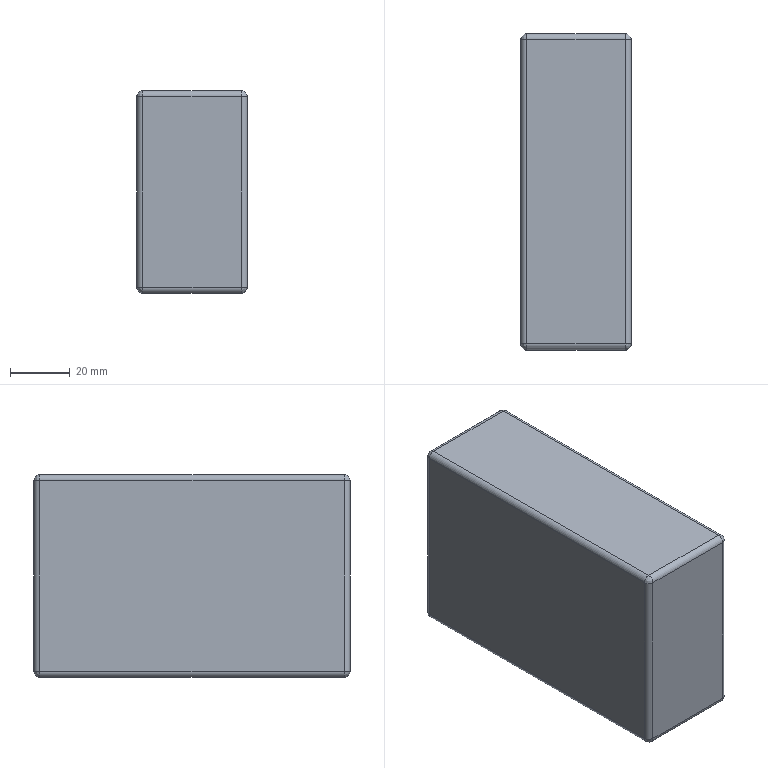Part | SolidWorks | features BaseBody 1 | 1 solid | 26 faces | box 37 x 106 x 68 mm | volume 265982 mm3 | cylinder 12 | spline 8 | plane 6 | commonest cylinder face diameters 4 x12
STEP:
#1=CARTESIAN_POINT('',(-18.5,-51.,-32.));
#2=VERTEX_POINT('',#1);
#3=CARTESIAN_POINT('',(-18.5,51.,-32.));
#4=VERTEX_POINT('',#3);
#5=CARTESIAN_POINT('',(-18.5,53.,-32.));
#6=DIRECTION('',(0.,1.,0.));
#7=VECTOR('',#6,1000.);
#8=LINE('',#5,#7);
#9=EDGE_CURVE('',#2,#4,#8,.T.);
#10=ORIENTED_EDGE('',*,*,#9,.F.);
#11=CARTESIAN_POINT('',(-18.5,-51.,32.));
#12=VERTEX_POINT('',#11);
#13=CARTESIAN_POINT('',(-18.5,-51.,-34.));
#14=DIRECTION('',(0.,0.,-1.));
#15=VECTOR('',#14,1000.);
#16=LINE('',#13,#15);
#17=EDGE_CURVE('',#12,#2,#16,.T.);
#18=ORIENTED_EDGE('',*,*,#17,.F.);
#19=CARTESIAN_POINT('',(-18.5,51.,32.));
#20=VERTEX_POINT('',#19);
#21=CARTESIAN_POINT('',(-18.5,53.,32.));
#22=DIRECTION('',(0.,-1.,0.));
#23=VECTOR('',#22,1000.);
#24=LINE('',#21,#23);
#25=EDGE_CURVE('',#20,#12,#24,.T.);
#26=ORIENTED_EDGE('',*,*,#25,.F.);
#27=CARTESIAN_POINT('',(-18.5,51.,-34.));
#28=DIRECTION('',(0.,0.,1.));
#29=VECTOR('',#28,1000.);
#30=LINE('',#27,#29);
#31=EDGE_CURVE('',#4,#20,#30,.T.);
#32=ORIENTED_EDGE('',*,*,#31,.F.);
#33=EDGE_LOOP('',(#10,#18,#26,#32));
#34=FACE_OUTER_BOUND('',#33,.T.);
#35=CARTESIAN_POINT('',(-18.5,53.,-34.));
#36=DIRECTION('',(1.,0.,0.));
#37=DIRECTION('',(0.,0.,-1.));
#38=AXIS2_PLACEMENT_3D('',#35,#36,#37);
#39=PLANE('',#38);
#40=ADVANCED_FACE('',(#34),#39,.F.);
#41=CARTESIAN_POINT('',(-16.5,53.,32.));
#42=VERTEX_POINT('',#41);
#43=CARTESIAN_POINT('',(-16.5,53.,-32.));
#44=VERTEX_POINT('',#43);
#45=CARTESIAN_POINT('',(-16.5,53.,0.));
#46=DIRECTION('',(0.,0.,-1.));
#47=VECTOR('',#46,1000.);
#48=LINE('',#45,#47);
#49=EDGE_CURVE('',#42,#44,#48,.T.);
#50=ORIENTED_EDGE('',*,*,#49,.T.);
#51=CARTESIAN_POINT('',(-16.5,51.,-32.));
#52=DIRECTION('',(0.,0.,1.));
#53=DIRECTION('',(1.,0.,0.));
#54=AXIS2_PLACEMENT_3D('',#51,#52,#53);
#55=CIRCLE('',#54,2.);
#56=EDGE_CURVE('',#44,#4,#55,.T.);
#57=ORIENTED_EDGE('',*,*,#56,.T.);
#58=ORIENTED_EDGE('',*,*,#31,.T.);
#59=CARTESIAN_POINT('',(-16.5,51.,32.));
#60=DIRECTION('',(0.,0.,-1.));
#61=DIRECTION('',(1.,0.,0.));
#62=AXIS2_PLACEMENT_3D('',#59,#60,#61);
#63=CIRCLE('',#62,2.);
#64=EDGE_CURVE('',#20,#42,#63,.T.);
#65=ORIENTED_EDGE('',*,*,#64,.T.);
#66=EDGE_LOOP('',(#50,#57,#58,#65));
#67=FACE_OUTER_BOUND('',#66,.T.);
#68=CARTESIAN_POINT('',(-16.5,51.,0.));
#69=DIRECTION('',(0.,0.,1.));
#70=DIRECTION('',(1.,0.,0.));
#71=AXIS2_PLACEMENT_3D('',#68,#69,#70);
#72=CYLINDRICAL_SURFACE('',#71,2.);
#73=ADVANCED_FACE('',(#67),#72,.T.);
#74=CARTESIAN_POINT('',(-16.5,51.,-34.));
#75=VERTEX_POINT('',#74);
#76=CARTESIAN_POINT('',(-16.5,51.,-32.));
#77=DIRECTION('',(0.,-1.,0.));
#78=DIRECTION('',(0.,0.,-1.));
#79=AXIS2_PLACEMENT_3D('',#76,#77,#78);
#80=CIRCLE('',#79,2.);
#81=EDGE_CURVE('',#4,#75,#80,.T.);
#82=ORIENTED_EDGE('',*,*,#81,.T.);
#83=CARTESIAN_POINT('',(-16.5,-51.,-34.));
#84=VERTEX_POINT('',#83);
#85=CARTESIAN_POINT('',(-16.5,53.,-34.));
#86=DIRECTION('',(0.,-1.,0.));
#87=VECTOR('',#86,1000.);
#88=LINE('',#85,#87);
#89=EDGE_CURVE('',#75,#84,#88,.T.);
#90=ORIENTED_EDGE('',*,*,#89,.T.);
#91=CARTESIAN_POINT('',(-16.5,-51.,-32.));
#92=DIRECTION('',(0.,1.,0.));
#93=DIRECTION('',(0.,0.,-1.));
#94=AXIS2_PLACEMENT_3D('',#91,#92,#93);
#95=CIRCLE('',#94,2.);
#96=EDGE_CURVE('',#84,#2,#95,.T.);
#97=ORIENTED_EDGE('',*,*,#96,.T.);
#98=ORIENTED_EDGE('',*,*,#9,.T.);
#99=EDGE_LOOP('',(#82,#90,#97,#98));
#100=FACE_OUTER_BOUND('',#99,.T.);
#101=CARTESIAN_POINT('',(-16.5,53.,-32.));
#102=DIRECTION('',(0.,-1.,0.));
#103=DIRECTION('',(0.,0.,-1.));
#104=AXIS2_PLACEMENT_3D('',#101,#102,#103);
#105=CYLINDRICAL_SURFACE('',#104,2.);
#106=ADVANCED_FACE('',(#100),#105,.T.);
#107=ORIENTED_EDGE('',*,*,#17,.T.);
#108=CARTESIAN_POINT('',(-16.5,-53.,-32.));
#109=VERTEX_POINT('',#108);
#110=CARTESIAN_POINT('',(-16.5,-51.,-32.));
#111=DIRECTION('',(0.,0.,1.));
#112=DIRECTION('',(-1.,0.,0.));
#113=AXIS2_PLACEMENT_3D('',#110,#111,#112);
#114=CIRCLE('',#113,2.);
#115=EDGE_CURVE('',#2,#109,#114,.T.);
#116=ORIENTED_EDGE('',*,*,#115,.T.);
#117=CARTESIAN_POINT('',(-16.5,-53.,32.));
#118=VERTEX_POINT('',#117);
#119=CARTESIAN_POINT('',(-16.5,-53.,-34.));
#120=DIRECTION('',(0.,0.,1.));
#121=VECTOR('',#120,1000.);
#122=LINE('',#119,#121);
#123=EDGE_CURVE('',#109,#118,#122,.T.);
#124=ORIENTED_EDGE('',*,*,#123,.T.);
#125=CARTESIAN_POINT('',(-16.5,-51.,32.));
#126=DIRECTION('',(0.,0.,-1.));
#127=DIRECTION('',(-1.,0.,0.));
#128=AXIS2_PLACEMENT_3D('',#125,#126,#127);
#129=CIRCLE('',#128,2.);
#130=EDGE_CURVE('',#118,#12,#129,.T.);
#131=ORIENTED_EDGE('',*,*,#130,.T.);
#132=EDGE_LOOP('',(#107,#116,#124,#131));
#133=FACE_OUTER_BOUND('',#132,.T.);
#134=CARTESIAN_POINT('',(-16.5,-51.,-34.));
#135=DIRECTION('',(0.,0.,-1.));
#136=DIRECTION('',(-1.,0.,0.));
#137=AXIS2_PLACEMENT_3D('',#134,#135,#136);
#138=CYLINDRICAL_SURFACE('',#137,2.);
#139=ADVANCED_FACE('',(#133),#138,.T.);
#140=CARTESIAN_POINT('',(-16.5,51.,34.));
#141=VERTEX_POINT('',#140);
#142=CARTESIAN_POINT('',(-16.5,51.,32.));
#143=DIRECTION('',(0.,-1.,0.));
#144=DIRECTION('',(0.,0.,-1.));
#145=AXIS2_PLACEMENT_3D('',#142,#143,#144);
#146=CIRCLE('',#145,2.);
#147=EDGE_CURVE('',#141,#20,#146,.T.);
#148=ORIENTED_EDGE('',*,*,#147,.T.);
#149=ORIENTED_EDGE('',*,*,#25,.T.);
#150=CARTESIAN_POINT('',(-16.5,-51.,34.));
#151=VERTEX_POINT('',#150);
#152=CARTESIAN_POINT('',(-16.5,-51.,32.));
#153=DIRECTION('',(0.,1.,0.));
#154=DIRECTION('',(0.,0.,-1.));
#155=AXIS2_PLACEMENT_3D('',#152,#153,#154);
#156=CIRCLE('',#155,2.);
#157=EDGE_CURVE('',#12,#151,#156,.T.);
#158=ORIENTED_EDGE('',*,*,#157,.T.);
#159=CARTESIAN_POINT('',(-16.5,53.,34.));
#160=DIRECTION('',(0.,1.,0.));
#161=VECTOR('',#160,1000.);
#162=LINE('',#159,#161);
#163=EDGE_CURVE('',#151,#141,#162,.T.);
#164=ORIENTED_EDGE('',*,*,#163,.T.);
#165=EDGE_LOOP('',(#148,#149,#158,#164));
#166=FACE_OUTER_BOUND('',#165,.T.);
#167=CARTESIAN_POINT('',(-16.5,53.,32.));
#168=DIRECTION('',(0.,-1.,0.));
#169=DIRECTION('',(0.,0.,-1.));
#170=AXIS2_PLACEMENT_3D('',#167,#168,#169);
#171=CYLINDRICAL_SURFACE('',#170,2.);
#172=ADVANCED_FACE('',(#166),#171,.T.);
#173=ORIENTED_EDGE('',*,*,#81,.F.);
#174=ORIENTED_EDGE('',*,*,#56,.F.);
#175=CARTESIAN_POINT('',(-16.5,51.,-32.));
#176=DIRECTION('',(-1.,0.,0.));
#177=DIRECTION('',(0.,0.,-1.));
#178=AXIS2_PLACEMENT_3D('',#175,#176,#177);
#179=CIRCLE('',#178,2.);
#180=EDGE_CURVE('',#44,#75,#179,.T.);
#181=ORIENTED_EDGE('',*,*,#180,.T.);
#182=EDGE_LOOP('',(#173,#174,#181));
#183=FACE_OUTER_BOUND('',#182,.T.);
#184=CARTESIAN_POINT('',(-16.5,51.,-34.));
#185=CARTESIAN_POINT('',(-16.5,51.,-34.));
#186=CARTESIAN_POINT('',(-16.5,51.,-34.));
#187=CARTESIAN_POINT('',(-16.5,51.,-34.));
#188=CARTESIAN_POINT('',(-17.672,51.,-34.));
#189=CARTESIAN_POINT('',(-17.672,51.686,-34.));
#190=CARTESIAN_POINT('',(-17.186,52.172,-34.));
#191=CARTESIAN_POINT('',(-16.5,52.172,-34.));
#192=CARTESIAN_POINT('',(-18.5,51.,-33.172));
#193=CARTESIAN_POINT('',(-18.5,52.172,-33.172));
#194=CARTESIAN_POINT('',(-17.672,53.,-33.172));
#195=CARTESIAN_POINT('',(-16.5,53.,-33.172));
#196=CARTESIAN_POINT('',(-18.5,51.,-32.));
#197=CARTESIAN_POINT('',(-18.5,52.172,-32.));
#198=CARTESIAN_POINT('',(-17.672,53.,-32.));
#199=CARTESIAN_POINT('',(-16.5,53.,-32.));
#200=(BOUNDED_SURFACE()B_SPLINE_SURFACE(3,3,((#184,#185,#186,#187),(#188,#189,#190,#191),(#192,#193,#194,#195),(#196,#197,#198,#199)),.UNSPECIFIED.,.F.,.F.,.F.)B_SPLINE_SURFACE_WITH_KNOTS((4,4),(4,4),(0.,1.),(0.,1.),.UNSPECIFIED.)GEOMETRIC_REPRESENTATION_ITEM()RATIONAL_B_SPLINE_SURFACE(((1.,0.8047,0.8047,1.),(0.8047,0.6476,0.6476,0.8047),(0.8047,0.6476,0.6476,0.8047),(1.,0.8047,0.8047,1.)))REPRESENTATION_ITEM('')SURFACE());
#201=ADVANCED_FACE('',(#183),#200,.T.);
#202=CARTESIAN_POINT('',(16.5,53.,-32.));
#203=VERTEX_POINT('',#202);
#204=CARTESIAN_POINT('',(0.,53.,-32.));
#205=DIRECTION('',(1.,0.,0.));
#206=VECTOR('',#205,1000.);
#207=LINE('',#204,#206);
#208=EDGE_CURVE('',#44,#203,#207,.T.);
#209=ORIENTED_EDGE('',*,*,#208,.F.);
#210=ORIENTED_EDGE('',*,*,#49,.F.);
#211=CARTESIAN_POINT('',(16.5,53.,32.));
#212=VERTEX_POINT('',#211);
#213=CARTESIAN_POINT('',(0.,53.,32.));
#214=DIRECTION('',(-1.,0.,0.));
#215=VECTOR('',#214,1000.);
#216=LINE('',#213,#215);
#217=EDGE_CURVE('',#212,#42,#216,.T.);
#218=ORIENTED_EDGE('',*,*,#217,.F.);
#219=CARTESIAN_POINT('',(16.5,53.,0.));
#220=DIRECTION('',(0.,0.,1.));
#221=VECTOR('',#220,1000.);
#222=LINE('',#219,#221);
#223=EDGE_CURVE('',#203,#212,#222,.T.);
#224=ORIENTED_EDGE('',*,*,#223,.F.);
#225=EDGE_LOOP('',(#209,#210,#218,#224));
#226=FACE_OUTER_BOUND('',#225,.T.);
#227=CARTESIAN_POINT('',(0.,53.,0.));
#228=DIRECTION('',(0.,-1.,0.));
#229=DIRECTION('',(0.,0.,-1.));
#230=AXIS2_PLACEMENT_3D('',#227,#228,#229);
#231=PLANE('',#230);
#232=ADVANCED_FACE('',(#226),#231,.F.);
#233=ORIENTED_EDGE('',*,*,#147,.F.);
#234=CARTESIAN_POINT('',(-16.5,51.,32.));
#235=DIRECTION('',(-1.,0.,0.));
#236=DIRECTION('',(0.,1.,0.));
#237=AXIS2_PLACEMENT_3D('',#234,#235,#236);
#238=CIRCLE('',#237,2.);
#239=EDGE_CURVE('',#141,#42,#238,.T.);
#240=ORIENTED_EDGE('',*,*,#239,.T.);
#241=ORIENTED_EDGE('',*,*,#64,.F.);
#242=EDGE_LOOP('',(#233,#240,#241));
#243=FACE_OUTER_BOUND('',#242,.T.);
#244=CARTESIAN_POINT('',(-16.5,53.,32.));
#245=CARTESIAN_POINT('',(-16.5,53.,32.));
#246=CARTESIAN_POINT('',(-16.5,53.,32.));
#247=CARTESIAN_POINT('',(-16.5,53.,32.));
#248=CARTESIAN_POINT('',(-17.672,53.,32.));
#249=CARTESIAN_POINT('',(-17.672,53.,32.686));
#250=CARTESIAN_POINT('',(-17.186,53.,33.172));
#251=CARTESIAN_POINT('',(-16.5,53.,33.172));
#252=CARTESIAN_POINT('',(-18.5,52.172,32.));
#253=CARTESIAN_POINT('',(-18.5,52.172,33.172));
#254=CARTESIAN_POINT('',(-17.672,52.172,34.));
#255=CARTESIAN_POINT('',(-16.5,52.172,34.));
#256=CARTESIAN_POINT('',(-18.5,51.,32.));
#257=CARTESIAN_POINT('',(-18.5,51.,33.172));
#258=CARTESIAN_POINT('',(-17.672,51.,34.));
#259=CARTESIAN_POINT('',(-16.5,51.,34.));
#260=(BOUNDED_SURFACE()B_SPLINE_SURFACE(3,3,((#244,#245,#246,#247),(#248,#249,#250,#251),(#252,#253,#254,#255),(#256,#257,#258,#259)),.UNSPECIFIED.,.F.,.F.,.T.)B_SPLINE_SURFACE_WITH_KNOTS((4,4),(4,4),(0.,1.),(0.,1.),.UNSPECIFIED.)GEOMETRIC_REPRESENTATION_ITEM()RATIONAL_B_SPLINE_SURFACE(((1.,0.8047,0.8047,1.),(0.8047,0.6476,0.6476,0.8047),(0.8047,0.6476,0.6476,0.8047),(1.,0.8047,0.8047,1.)))REPRESENTATION_ITEM('')SURFACE());
#261=ADVANCED_FACE('',(#243),#260,.T.);
#262=CARTESIAN_POINT('',(16.5,-51.,-34.));
#263=VERTEX_POINT('',#262);
#264=CARTESIAN_POINT('',(16.5,51.,-34.));
#265=VERTEX_POINT('',#264);
#266=CARTESIAN_POINT('',(16.5,53.,-34.));
#267=DIRECTION('',(0.,1.,0.));
#268=VECTOR('',#267,1000.);
#269=LINE('',#266,#268);
#270=EDGE_CURVE('',#263,#265,#269,.T.);
#271=ORIENTED_EDGE('',*,*,#270,.F.);
#272=CARTESIAN_POINT('',(18.5,-51.,-34.));
#273=DIRECTION('',(1.,0.,0.));
#274=VECTOR('',#273,1000.);
#275=LINE('',#272,#274);
#276=EDGE_CURVE('',#84,#263,#275,.T.);
#277=ORIENTED_EDGE('',*,*,#276,.F.);
#278=ORIENTED_EDGE('',*,*,#89,.F.);
#279=CARTESIAN_POINT('',(18.5,51.,-34.));
#280=DIRECTION('',(-1.,0.,0.));
#281=VECTOR('',#280,1000.);
#282=LINE('',#279,#281);
#283=EDGE_CURVE('',#265,#75,#282,.T.);
#284=ORIENTED_EDGE('',*,*,#283,.F.);
#285=EDGE_LOOP('',(#271,#277,#278,#284));
#286=FACE_OUTER_BOUND('',#285,.T.);
#287=CARTESIAN_POINT('',(18.5,53.,-34.));
#288=DIRECTION('',(0.,0.,1.));
#289=DIRECTION('',(1.,0.,0.));
#290=AXIS2_PLACEMENT_3D('',#287,#288,#289);
#291=PLANE('',#290);
#292=ADVANCED_FACE('',(#286),#291,.F.);
#293=CARTESIAN_POINT('',(-16.5,-51.,-32.));
#294=DIRECTION('',(-1.,0.,0.));
#295=DIRECTION('',(0.,-1.,0.));
#296=AXIS2_PLACEMENT_3D('',#293,#294,#295);
#297=CIRCLE('',#296,2.);
#298=EDGE_CURVE('',#84,#109,#297,.T.);
#299=ORIENTED_EDGE('',*,*,#298,.T.);
#300=ORIENTED_EDGE('',*,*,#115,.F.);
#301=ORIENTED_EDGE('',*,*,#96,.F.);
#302=EDGE_LOOP('',(#299,#300,#301));
#303=FACE_OUTER_BOUND('',#302,.T.);
#304=CARTESIAN_POINT('',(-16.5,-53.,-32.));
#305=CARTESIAN_POINT('',(-16.5,-53.,-32.));
#306=CARTESIAN_POINT('',(-16.5,-53.,-32.));
#307=CARTESIAN_POINT('',(-16.5,-53.,-32.));
#308=CARTESIAN_POINT('',(-17.672,-53.,-32.));
#309=CARTESIAN_POINT('',(-17.672,-53.,-32.686));
#310=CARTESIAN_POINT('',(-17.186,-53.,-33.172));
#311=CARTESIAN_POINT('',(-16.5,-53.,-33.172));
#312=CARTESIAN_POINT('',(-18.5,-52.172,-32.));
#313=CARTESIAN_POINT('',(-18.5,-52.172,-33.172));
#314=CARTESIAN_POINT('',(-17.672,-52.172,-34.));
#315=CARTESIAN_POINT('',(-16.5,-52.172,-34.));
#316=CARTESIAN_POINT('',(-18.5,-51.,-32.));
#317=CARTESIAN_POINT('',(-18.5,-51.,-33.172));
#318=CARTESIAN_POINT('',(-17.672,-51.,-34.));
#319=CARTESIAN_POINT('',(-16.5,-51.,-34.));
#320=(BOUNDED_SURFACE()B_SPLINE_SURFACE(3,3,((#304,#305,#306,#307),(#308,#309,#310,#311),(#312,#313,#314,#315),(#316,#317,#318,#319)),.UNSPECIFIED.,.F.,.F.,.T.)B_SPLINE_SURFACE_WITH_KNOTS((4,4),(4,4),(0.,1.),(0.,1.),.UNSPECIFIED.)GEOMETRIC_REPRESENTATION_ITEM()RATIONAL_B_SPLINE_SURFACE(((1.,0.8047,0.8047,1.),(0.8047,0.6476,0.6476,0.8047),(0.8047,0.6476,0.6476,0.8047),(1.,0.8047,0.8047,1.)))REPRESENTATION_ITEM('')SURFACE());
#321=ADVANCED_FACE('',(#303),#320,.T.);
#322=ORIENTED_EDGE('',*,*,#157,.F.);
#323=ORIENTED_EDGE('',*,*,#130,.F.);
#324=CARTESIAN_POINT('',(-16.5,-51.,32.));
#325=DIRECTION('',(-1.,0.,0.));
#326=DIRECTION('',(0.,0.,1.));
#327=AXIS2_PLACEMENT_3D('',#324,#325,#326);
#328=CIRCLE('',#327,2.);
#329=EDGE_CURVE('',#118,#151,#328,.T.);
#330=ORIENTED_EDGE('',*,*,#329,.T.);
#331=EDGE_LOOP('',(#322,#323,#330));
#332=FACE_OUTER_BOUND('',#331,.T.);
#333=CARTESIAN_POINT('',(-16.5,-51.,34.));
#334=CARTESIAN_POINT('',(-16.5,-51.,34.));
#335=CARTESIAN_POINT('',(-16.5,-51.,34.));
#336=CARTESIAN_POINT('',(-16.5,-51.,34.));
#337=CARTESIAN_POINT('',(-17.672,-51.,34.));
#338=CARTESIAN_POINT('',(-17.672,-51.686,34.));
#339=CARTESIAN_POINT('',(-17.186,-52.172,34.));
#340=CARTESIAN_POINT('',(-16.5,-52.172,34.));
#341=CARTESIAN_POINT('',(-18.5,-51.,33.172));
#342=CARTESIAN_POINT('',(-18.5,-52.172,33.172));
#343=CARTESIAN_POINT('',(-17.672,-53.,33.172));
#344=CARTESIAN_POINT('',(-16.5,-53.,33.172));
#345=CARTESIAN_POINT('',(-18.5,-51.,32.));
#346=CARTESIAN_POINT('',(-18.5,-52.172,32.));
#347=CARTESIAN_POINT('',(-17.672,-53.,32.));
#348=CARTESIAN_POINT('',(-16.5,-53.,32.));
#349=(BOUNDED_SURFACE()B_SPLINE_SURFACE(3,3,((#333,#334,#335,#336),(#337,#338,#339,#340),(#341,#342,#343,#344),(#345,#346,#347,#348)),.UNSPECIFIED.,.F.,.F.,.F.)B_SPLINE_SURFACE_WITH_KNOTS((4,4),(4,4),(0.,1.),(0.,1.),.UNSPECIFIED.)GEOMETRIC_REPRESENTATION_ITEM()RATIONAL_B_SPLINE_SURFACE(((1.,0.8047,0.8047,1.),(0.8047,0.6476,0.6476,0.8047),(0.8047,0.6476,0.6476,0.8047),(1.,0.8047,0.8047,1.)))REPRESENTATION_ITEM('')SURFACE());
#350=ADVANCED_FACE('',(#332),#349,.T.);
#351=CARTESIAN_POINT('',(16.5,-53.,-32.));
#352=VERTEX_POINT('',#351);
#353=CARTESIAN_POINT('',(16.5,-53.,32.));
#354=VERTEX_POINT('',#353);
#355=CARTESIAN_POINT('',(16.5,-53.,0.));
#356=DIRECTION('',(0.,0.,1.));
#357=VECTOR('',#356,1000.);
#358=LINE('',#355,#357);
#359=EDGE_CURVE('',#352,#354,#358,.T.);
#360=ORIENTED_EDGE('',*,*,#359,.T.);
#361=CARTESIAN_POINT('',(0.,-53.,32.));
#362=DIRECTION('',(-1.,0.,0.));
#363=VECTOR('',#362,1000.);
#364=LINE('',#361,#363);
#365=EDGE_CURVE('',#354,#118,#364,.T.);
#366=ORIENTED_EDGE('',*,*,#365,.T.);
#367=ORIENTED_EDGE('',*,*,#123,.F.);
#368=CARTESIAN_POINT('',(0.,-53.,-32.));
#369=DIRECTION('',(1.,0.,0.));
#370=VECTOR('',#369,1000.);
#371=LINE('',#368,#370);
#372=EDGE_CURVE('',#109,#352,#371,.T.);
#373=ORIENTED_EDGE('',*,*,#372,.T.);
#374=EDGE_LOOP('',(#360,#366,#367,#373));
#375=FACE_OUTER_BOUND('',#374,.T.);
#376=CARTESIAN_POINT('',(0.,-53.,0.));
#377=DIRECTION('',(0.,-1.,0.));
#378=DIRECTION('',(0.,0.,-1.));
#379=AXIS2_PLACEMENT_3D('',#376,#377,#378);
#380=PLANE('',#379);
#381=ADVANCED_FACE('',(#375),#380,.T.);
#382=ORIENTED_EDGE('',*,*,#163,.F.);
#383=CARTESIAN_POINT('',(16.5,-51.,34.));
#384=VERTEX_POINT('',#383);
#385=CARTESIAN_POINT('',(18.5,-51.,34.));
#386=DIRECTION('',(-1.,0.,0.));
#387=VECTOR('',#386,1000.);
#388=LINE('',#385,#387);
#389=EDGE_CURVE('',#384,#151,#388,.T.);
#390=ORIENTED_EDGE('',*,*,#389,.F.);
#391=CARTESIAN_POINT('',(16.5,51.,34.));
#392=VERTEX_POINT('',#391);
#393=CARTESIAN_POINT('',(16.5,53.,34.));
#394=DIRECTION('',(0.,-1.,0.));
#395=VECTOR('',#394,1000.);
#396=LINE('',#393,#395);
#397=EDGE_CURVE('',#392,#384,#396,.T.);
#398=ORIENTED_EDGE('',*,*,#397,.F.);
#399=CARTESIAN_POINT('',(18.5,51.,34.));
#400=DIRECTION('',(1.,0.,0.));
#401=VECTOR('',#400,1000.);
#402=LINE('',#399,#401);
#403=EDGE_CURVE('',#141,#392,#402,.T.);
#404=ORIENTED_EDGE('',*,*,#403,.F.);
#405=EDGE_LOOP('',(#382,#390,#398,#404));
#406=FACE_OUTER_BOUND('',#405,.T.);
#407=CARTESIAN_POINT('',(18.5,53.,34.));
#408=DIRECTION('',(0.,0.,-1.));
#409=DIRECTION('',(-1.,0.,0.));
#410=AXIS2_PLACEMENT_3D('',#407,#408,#409);
#411=PLANE('',#410);
#412=ADVANCED_FACE('',(#406),#411,.F.);
#413=ORIENTED_EDGE('',*,*,#208,.T.);
#414=CARTESIAN_POINT('',(16.5,51.,-32.));
#415=DIRECTION('',(-1.,0.,0.));
#416=DIRECTION('',(0.,0.,1.));
#417=AXIS2_PLACEMENT_3D('',#414,#415,#416);
#418=CIRCLE('',#417,2.);
#419=EDGE_CURVE('',#203,#265,#418,.T.);
#420=ORIENTED_EDGE('',*,*,#419,.T.);
#421=ORIENTED_EDGE('',*,*,#283,.T.);
#422=ORIENTED_EDGE('',*,*,#180,.F.);
#423=EDGE_LOOP('',(#413,#420,#421,#422));
#424=FACE_OUTER_BOUND('',#423,.T.);
#425=CARTESIAN_POINT('',(0.,51.,-32.));
#426=DIRECTION('',(-1.,0.,0.));
#427=DIRECTION('',(0.,0.,1.));
#428=AXIS2_PLACEMENT_3D('',#425,#426,#427);
#429=CYLINDRICAL_SURFACE('',#428,2.);
#430=ADVANCED_FACE('',(#424),#429,.T.);
#431=CARTESIAN_POINT('',(18.5,51.,32.));
#432=VERTEX_POINT('',#431);
#433=CARTESIAN_POINT('',(18.5,51.,-32.));
#434=VERTEX_POINT('',#433);
#435=CARTESIAN_POINT('',(18.5,51.,0.));
#436=DIRECTION('',(0.,0.,-1.));
#437=VECTOR('',#436,1000.);
#438=LINE('',#435,#437);
#439=EDGE_CURVE('',#432,#434,#438,.T.);
#440=ORIENTED_EDGE('',*,*,#439,.T.);
#441=CARTESIAN_POINT('',(16.5,51.,-32.));
#442=DIRECTION('',(0.,0.,1.));
#443=DIRECTION('',(-1.,0.,0.));
#444=AXIS2_PLACEMENT_3D('',#441,#442,#443);
#445=CIRCLE('',#444,2.);
#446=EDGE_CURVE('',#434,#203,#445,.T.);
#447=ORIENTED_EDGE('',*,*,#446,.T.);
#448=ORIENTED_EDGE('',*,*,#223,.T.);
#449=CARTESIAN_POINT('',(16.5,51.,32.));
#450=DIRECTION('',(0.,0.,-1.));
#451=DIRECTION('',(-1.,0.,0.));
#452=AXIS2_PLACEMENT_3D('',#449,#450,#451);
#453=CIRCLE('',#452,2.);
#454=EDGE_CURVE('',#212,#432,#453,.T.);
#455=ORIENTED_EDGE('',*,*,#454,.T.);
#456=EDGE_LOOP('',(#440,#447,#448,#455));
#457=FACE_OUTER_BOUND('',#456,.T.);
#458=CARTESIAN_POINT('',(16.5,51.,0.));
#459=DIRECTION('',(0.,0.,-1.));
#460=DIRECTION('',(-1.,0.,0.));
#461=AXIS2_PLACEMENT_3D('',#458,#459,#460);
#462=CYLINDRICAL_SURFACE('',#461,2.);
#463=ADVANCED_FACE('',(#457),#462,.T.);
#464=ORIENTED_EDGE('',*,*,#403,.T.);
#465=CARTESIAN_POINT('',(16.5,51.,32.));
#466=DIRECTION('',(-1.,0.,0.));
#467=DIRECTION('',(0.,0.,-1.));
#468=AXIS2_PLACEMENT_3D('',#465,#466,#467);
#469=CIRCLE('',#468,2.);
#470=EDGE_CURVE('',#392,#212,#469,.T.);
#471=ORIENTED_EDGE('',*,*,#470,.T.);
#472=ORIENTED_EDGE('',*,*,#217,.T.);
#473=ORIENTED_EDGE('',*,*,#239,.F.);
#474=EDGE_LOOP('',(#464,#471,#472,#473));
#475=FACE_OUTER_BOUND('',#474,.T.);
#476=CARTESIAN_POINT('',(0.,51.,32.));
#477=DIRECTION('',(1.,0.,0.));
#478=DIRECTION('',(0.,0.,-1.));
#479=AXIS2_PLACEMENT_3D('',#476,#477,#478);
#480=CYLINDRICAL_SURFACE('',#479,2.);
#481=ADVANCED_FACE('',(#475),#480,.T.);
#482=CARTESIAN_POINT('',(16.5,51.,-32.));
#483=DIRECTION('',(0.,-1.,0.));
#484=DIRECTION('',(0.,0.,-1.));
#485=AXIS2_PLACEMENT_3D('',#482,#483,#484);
#486=CIRCLE('',#485,2.);
#487=EDGE_CURVE('',#265,#434,#486,.T.);
#488=ORIENTED_EDGE('',*,*,#487,.T.);
#489=CARTESIAN_POINT('',(18.5,-51.,-32.));
#490=VERTEX_POINT('',#489);
#491=CARTESIAN_POINT('',(18.5,53.,-32.));
#492=DIRECTION('',(0.,-1.,0.));
#493=VECTOR('',#492,1000.);
#494=LINE('',#491,#493);
#495=EDGE_CURVE('',#434,#490,#494,.T.);
#496=ORIENTED_EDGE('',*,*,#495,.T.);
#497=CARTESIAN_POINT('',(16.5,-51.,-32.));
#498=DIRECTION('',(0.,1.,0.));
#499=DIRECTION('',(0.,0.,-1.));
#500=AXIS2_PLACEMENT_3D('',#497,#498,#499);
#501=CIRCLE('',#500,2.);
#502=EDGE_CURVE('',#490,#263,#501,.T.);
#503=ORIENTED_EDGE('',*,*,#502,.T.);
#504=ORIENTED_EDGE('',*,*,#270,.T.);
#505=EDGE_LOOP('',(#488,#496,#503,#504));
#506=FACE_OUTER_BOUND('',#505,.T.);
#507=CARTESIAN_POINT('',(16.5,53.,-32.));
#508=DIRECTION('',(0.,-1.,0.));
#509=DIRECTION('',(0.,0.,-1.));
#510=AXIS2_PLACEMENT_3D('',#507,#508,#509);
#511=CYLINDRICAL_SURFACE('',#510,2.);
#512=ADVANCED_FACE('',(#506),#511,.T.);
#513=ORIENTED_EDGE('',*,*,#276,.T.);
#514=CARTESIAN_POINT('',(16.5,-51.,-32.));
#515=DIRECTION('',(-1.,0.,0.));
#516=DIRECTION('',(0.,0.,-1.));
#517=AXIS2_PLACEMENT_3D('',#514,#515,#516);
#518=CIRCLE('',#517,2.);
#519=EDGE_CURVE('',#263,#352,#518,.T.);
#520=ORIENTED_EDGE('',*,*,#519,.T.);
#521=ORIENTED_EDGE('',*,*,#372,.F.);
#522=ORIENTED_EDGE('',*,*,#298,.F.);
#523=EDGE_LOOP('',(#513,#520,#521,#522));
#524=FACE_OUTER_BOUND('',#523,.T.);
#525=CARTESIAN_POINT('',(18.5,-51.,-32.));
#526=DIRECTION('',(1.,0.,0.));
#527=DIRECTION('',(0.,0.,-1.));
#528=AXIS2_PLACEMENT_3D('',#525,#526,#527);
#529=CYLINDRICAL_SURFACE('',#528,2.);
#530=ADVANCED_FACE('',(#524),#529,.T.);
#531=ORIENTED_EDGE('',*,*,#365,.F.);
#532=CARTESIAN_POINT('',(16.5,-51.,32.));
#533=DIRECTION('',(-1.,0.,0.));
#534=DIRECTION('',(0.,0.,1.));
#535=AXIS2_PLACEMENT_3D('',#532,#533,#534);
#536=CIRCLE('',#535,2.);
#537=EDGE_CURVE('',#354,#384,#536,.T.);
#538=ORIENTED_EDGE('',*,*,#537,.T.);
#539=ORIENTED_EDGE('',*,*,#389,.T.);
#540=ORIENTED_EDGE('',*,*,#329,.F.);
#541=EDGE_LOOP('',(#531,#538,#539,#540));
#542=FACE_OUTER_BOUND('',#541,.T.);
#543=CARTESIAN_POINT('',(18.5,-51.,32.));
#544=DIRECTION('',(-1.,0.,0.));
#545=DIRECTION('',(0.,0.,1.));
#546=AXIS2_PLACEMENT_3D('',#543,#544,#545);
#547=CYLINDRICAL_SURFACE('',#546,2.);
#548=ADVANCED_FACE('',(#542),#547,.T.);
#549=ORIENTED_EDGE('',*,*,#359,.F.);
#550=CARTESIAN_POINT('',(16.5,-51.,-32.));
#551=DIRECTION('',(0.,0.,1.));
#552=DIRECTION('',(1.,0.,0.));
#553=AXIS2_PLACEMENT_3D('',#550,#551,#552);
#554=CIRCLE('',#553,2.);
#555=EDGE_CURVE('',#352,#490,#554,.T.);
#556=ORIENTED_EDGE('',*,*,#555,.T.);
#557=CARTESIAN_POINT('',(18.5,-51.,32.));
#558=VERTEX_POINT('',#557);
#559=CARTESIAN_POINT('',(18.5,-51.,-34.));
#560=DIRECTION('',(0.,0.,1.));
#561=VECTOR('',#560,1000.);
#562=LINE('',#559,#561);
#563=EDGE_CURVE('',#490,#558,#562,.T.);
#564=ORIENTED_EDGE('',*,*,#563,.T.);
#565=CARTESIAN_POINT('',(16.5,-51.,32.));
#566=DIRECTION('',(0.,0.,-1.));
#567=DIRECTION('',(1.,0.,0.));
#568=AXIS2_PLACEMENT_3D('',#565,#566,#567);
#569=CIRCLE('',#568,2.);
#570=EDGE_CURVE('',#558,#354,#569,.T.);
#571=ORIENTED_EDGE('',*,*,#570,.T.);
#572=EDGE_LOOP('',(#549,#556,#564,#571));
#573=FACE_OUTER_BOUND('',#572,.T.);
#574=CARTESIAN_POINT('',(16.5,-51.,-34.));
#575=DIRECTION('',(0.,0.,1.));
#576=DIRECTION('',(1.,0.,0.));
#577=AXIS2_PLACEMENT_3D('',#574,#575,#576);
#578=CYLINDRICAL_SURFACE('',#577,2.);
#579=ADVANCED_FACE('',(#573),#578,.T.);
#580=CARTESIAN_POINT('',(16.5,51.,32.));
#581=DIRECTION('',(0.,-1.,0.));
#582=DIRECTION('',(0.,0.,-1.));
#583=AXIS2_PLACEMENT_3D('',#580,#581,#582);
#584=CIRCLE('',#583,2.);
#585=EDGE_CURVE('',#432,#392,#584,.T.);
#586=ORIENTED_EDGE('',*,*,#585,.T.);
#587=ORIENTED_EDGE('',*,*,#397,.T.);
#588=CARTESIAN_POINT('',(16.5,-51.,32.));
#589=DIRECTION('',(0.,1.,0.));
#590=DIRECTION('',(0.,0.,-1.));
#591=AXIS2_PLACEMENT_3D('',#588,#589,#590);
#592=CIRCLE('',#591,2.);
#593=EDGE_CURVE('',#384,#558,#592,.T.);
#594=ORIENTED_EDGE('',*,*,#593,.T.);
#595=CARTESIAN_POINT('',(18.5,53.,32.));
#596=DIRECTION('',(0.,1.,0.));
#597=VECTOR('',#596,1000.);
#598=LINE('',#595,#597);
#599=EDGE_CURVE('',#558,#432,#598,.T.);
#600=ORIENTED_EDGE('',*,*,#599,.T.);
#601=EDGE_LOOP('',(#586,#587,#594,#600));
#602=FACE_OUTER_BOUND('',#601,.T.);
#603=CARTESIAN_POINT('',(16.5,53.,32.));
#604=DIRECTION('',(0.,-1.,0.));
#605=DIRECTION('',(0.,0.,-1.));
#606=AXIS2_PLACEMENT_3D('',#603,#604,#605);
#607=CYLINDRICAL_SURFACE('',#606,2.);
#608=ADVANCED_FACE('',(#602),#607,.T.);
#609=ORIENTED_EDGE('',*,*,#487,.F.);
#610=ORIENTED_EDGE('',*,*,#419,.F.);
#611=ORIENTED_EDGE('',*,*,#446,.F.);
#612=EDGE_LOOP('',(#609,#610,#611));
#613=FACE_OUTER_BOUND('',#612,.T.);
#614=CARTESIAN_POINT('',(18.5,51.,-32.));
#615=CARTESIAN_POINT('',(18.5,52.172,-32.));
#616=CARTESIAN_POINT('',(17.672,53.,-32.));
#617=CARTESIAN_POINT('',(16.5,53.,-32.));
#618=CARTESIAN_POINT('',(18.5,51.,-33.172));
#619=CARTESIAN_POINT('',(18.5,52.172,-33.172));
#620=CARTESIAN_POINT('',(17.672,53.,-33.172));
#621=CARTESIAN_POINT('',(16.5,53.,-33.172));
#622=CARTESIAN_POINT('',(17.672,51.,-34.));
#623=CARTESIAN_POINT('',(17.672,51.686,-34.));
#624=CARTESIAN_POINT('',(17.186,52.172,-34.));
#625=CARTESIAN_POINT('',(16.5,52.172,-34.));
#626=CARTESIAN_POINT('',(16.5,51.,-34.));
#627=CARTESIAN_POINT('',(16.5,51.,-34.));
#628=CARTESIAN_POINT('',(16.5,51.,-34.));
#629=CARTESIAN_POINT('',(16.5,51.,-34.));
#630=(BOUNDED_SURFACE()B_SPLINE_SURFACE(3,3,((#614,#615,#616,#617),(#618,#619,#620,#621),(#622,#623,#624,#625),(#626,#627,#628,#629)),.UNSPECIFIED.,.F.,.F.,.F.)B_SPLINE_SURFACE_WITH_KNOTS((4,4),(4,4),(0.,1.),(0.,1.),.UNSPECIFIED.)GEOMETRIC_REPRESENTATION_ITEM()RATIONAL_B_SPLINE_SURFACE(((1.,0.8047,0.8047,1.),(0.8047,0.6476,0.6476,0.8047),(0.8047,0.6476,0.6476,0.8047),(1.,0.8047,0.8047,1.)))REPRESENTATION_ITEM('')SURFACE());
#631=ADVANCED_FACE('',(#613),#630,.T.);
#632=ORIENTED_EDGE('',*,*,#599,.F.);
#633=ORIENTED_EDGE('',*,*,#563,.F.);
#634=ORIENTED_EDGE('',*,*,#495,.F.);
#635=ORIENTED_EDGE('',*,*,#439,.F.);
#636=EDGE_LOOP('',(#632,#633,#634,#635));
#637=FACE_OUTER_BOUND('',#636,.T.);
#638=CARTESIAN_POINT('',(18.5,53.,-34.));
#639=DIRECTION('',(-1.,0.,0.));
#640=DIRECTION('',(0.,0.,1.));
#641=AXIS2_PLACEMENT_3D('',#638,#639,#640);
#642=PLANE('',#641);
#643=ADVANCED_FACE('',(#637),#642,.F.);
#644=ORIENTED_EDGE('',*,*,#454,.F.);
#645=ORIENTED_EDGE('',*,*,#470,.F.);
#646=ORIENTED_EDGE('',*,*,#585,.F.);
#647=EDGE_LOOP('',(#644,#645,#646));
#648=FACE_OUTER_BOUND('',#647,.T.);
#649=CARTESIAN_POINT('',(16.5,53.,32.));
#650=CARTESIAN_POINT('',(16.5,53.,32.));
#651=CARTESIAN_POINT('',(16.5,53.,32.));
#652=CARTESIAN_POINT('',(16.5,53.,32.));
#653=CARTESIAN_POINT('',(16.5,53.,33.172));
#654=CARTESIAN_POINT('',(17.186,53.,33.172));
#655=CARTESIAN_POINT('',(17.672,53.,32.686));
#656=CARTESIAN_POINT('',(17.672,53.,32.));
#657=CARTESIAN_POINT('',(16.5,52.172,34.));
#658=CARTESIAN_POINT('',(17.672,52.172,34.));
#659=CARTESIAN_POINT('',(18.5,52.172,33.172));
#660=CARTESIAN_POINT('',(18.5,52.172,32.));
#661=CARTESIAN_POINT('',(16.5,51.,34.));
#662=CARTESIAN_POINT('',(17.672,51.,34.));
#663=CARTESIAN_POINT('',(18.5,51.,33.172));
#664=CARTESIAN_POINT('',(18.5,51.,32.));
#665=(BOUNDED_SURFACE()B_SPLINE_SURFACE(3,3,((#649,#650,#651,#652),(#653,#654,#655,#656),(#657,#658,#659,#660),(#661,#662,#663,#664)),.UNSPECIFIED.,.F.,.F.,.F.)B_SPLINE_SURFACE_WITH_KNOTS((4,4),(4,4),(0.,1.),(0.,1.),.UNSPECIFIED.)GEOMETRIC_REPRESENTATION_ITEM()RATIONAL_B_SPLINE_SURFACE(((1.,0.8047,0.8047,1.),(0.8047,0.6476,0.6476,0.8047),(0.8047,0.6476,0.6476,0.8047),(1.,0.8047,0.8047,1.)))REPRESENTATION_ITEM('')SURFACE());
#666=ADVANCED_FACE('',(#648),#665,.T.);
#667=ORIENTED_EDGE('',*,*,#502,.F.);
#668=ORIENTED_EDGE('',*,*,#555,.F.);
#669=ORIENTED_EDGE('',*,*,#519,.F.);
#670=EDGE_LOOP('',(#667,#668,#669));
#671=FACE_OUTER_BOUND('',#670,.T.);
#672=CARTESIAN_POINT('',(18.5,-51.,-32.));
#673=CARTESIAN_POINT('',(18.5,-51.,-33.172));
#674=CARTESIAN_POINT('',(17.672,-51.,-34.));
#675=CARTESIAN_POINT('',(16.5,-51.,-34.));
#676=CARTESIAN_POINT('',(18.5,-52.172,-32.));
#677=CARTESIAN_POINT('',(18.5,-52.172,-33.172));
#678=CARTESIAN_POINT('',(17.672,-52.172,-34.));
#679=CARTESIAN_POINT('',(16.5,-52.172,-34.));
#680=CARTESIAN_POINT('',(17.672,-53.,-32.));
#681=CARTESIAN_POINT('',(17.672,-53.,-32.686));
#682=CARTESIAN_POINT('',(17.186,-53.,-33.172));
#683=CARTESIAN_POINT('',(16.5,-53.,-33.172));
#684=CARTESIAN_POINT('',(16.5,-53.,-32.));
#685=CARTESIAN_POINT('',(16.5,-53.,-32.));
#686=CARTESIAN_POINT('',(16.5,-53.,-32.));
#687=CARTESIAN_POINT('',(16.5,-53.,-32.));
#688=(BOUNDED_SURFACE()B_SPLINE_SURFACE(3,3,((#672,#673,#674,#675),(#676,#677,#678,#679),(#680,#681,#682,#683),(#684,#685,#686,#687)),.UNSPECIFIED.,.F.,.F.,.F.)B_SPLINE_SURFACE_WITH_KNOTS((4,4),(4,4),(0.,1.),(0.,1.),.UNSPECIFIED.)GEOMETRIC_REPRESENTATION_ITEM()RATIONAL_B_SPLINE_SURFACE(((1.,0.8047,0.8047,1.),(0.8047,0.6476,0.6476,0.8047),(0.8047,0.6476,0.6476,0.8047),(1.,0.8047,0.8047,1.)))REPRESENTATION_ITEM('')SURFACE());
#689=ADVANCED_FACE('',(#671),#688,.T.);
#690=ORIENTED_EDGE('',*,*,#593,.F.);
#691=ORIENTED_EDGE('',*,*,#537,.F.);
#692=ORIENTED_EDGE('',*,*,#570,.F.);
#693=EDGE_LOOP('',(#690,#691,#692));
#694=FACE_OUTER_BOUND('',#693,.T.);
#695=CARTESIAN_POINT('',(18.5,-51.,32.));
#696=CARTESIAN_POINT('',(18.5,-52.172,32.));
#697=CARTESIAN_POINT('',(17.672,-53.,32.));
#698=CARTESIAN_POINT('',(16.5,-53.,32.));
#699=CARTESIAN_POINT('',(18.5,-51.,33.172));
#700=CARTESIAN_POINT('',(18.5,-52.172,33.172));
#701=CARTESIAN_POINT('',(17.672,-53.,33.172));
#702=CARTESIAN_POINT('',(16.5,-53.,33.172));
#703=CARTESIAN_POINT('',(17.672,-51.,34.));
#704=CARTESIAN_POINT('',(17.672,-51.686,34.));
#705=CARTESIAN_POINT('',(17.186,-52.172,34.));
#706=CARTESIAN_POINT('',(16.5,-52.172,34.));
#707=CARTESIAN_POINT('',(16.5,-51.,34.));
#708=CARTESIAN_POINT('',(16.5,-51.,34.));
#709=CARTESIAN_POINT('',(16.5,-51.,34.));
#710=CARTESIAN_POINT('',(16.5,-51.,34.));
#711=(BOUNDED_SURFACE()B_SPLINE_SURFACE(3,3,((#695,#696,#697,#698),(#699,#700,#701,#702),(#703,#704,#705,#706),(#707,#708,#709,#710)),.UNSPECIFIED.,.F.,.F.,.T.)B_SPLINE_SURFACE_WITH_KNOTS((4,4),(4,4),(0.,1.),(0.,1.),.UNSPECIFIED.)GEOMETRIC_REPRESENTATION_ITEM()RATIONAL_B_SPLINE_SURFACE(((1.,0.8047,0.8047,1.),(0.8047,0.6476,0.6476,0.8047),(0.8047,0.6476,0.6476,0.8047),(1.,0.8047,0.8047,1.)))REPRESENTATION_ITEM('')SURFACE());
#712=ADVANCED_FACE('',(#694),#711,.T.);
#713=CLOSED_SHELL('',(#40,#73,#106,#139,#172,#201,#232,#261,#292,#321,#350,#381,#412,#430,#463,#481,#512,#530,#548,#579,#608,#631,#643,#666,#689,#712));
#714=MANIFOLD_SOLID_BREP('',#713);
#715=CARTESIAN_POINT('',(0.,0.,0.));
#716=DIRECTION('',(0.,0.,1.));
#717=DIRECTION('',(1.,0.,0.));
#718=AXIS2_PLACEMENT_3D('',#715,#716,#717);
#719=(LENGTH_UNIT()NAMED_UNIT(*)SI_UNIT(.MILLI.,.METRE.));
#720=UNCERTAINTY_MEASURE_WITH_UNIT(LENGTH_MEASURE(0.00001),#719,'','');
#721=(NAMED_UNIT(*)PLANE_ANGLE_UNIT()SI_UNIT($,.RADIAN.));
#722=(NAMED_UNIT(*)SI_UNIT($,.STERADIAN.)SOLID_ANGLE_UNIT());
#723=(GEOMETRIC_REPRESENTATION_CONTEXT(3)GLOBAL_UNCERTAINTY_ASSIGNED_CONTEXT((#720))GLOBAL_UNIT_ASSIGNED_CONTEXT((#719,#721,#722))REPRESENTATION_CONTEXT('',''));
#724=ADVANCED_BREP_SHAPE_REPRESENTATION('',(#714,#718),#723);